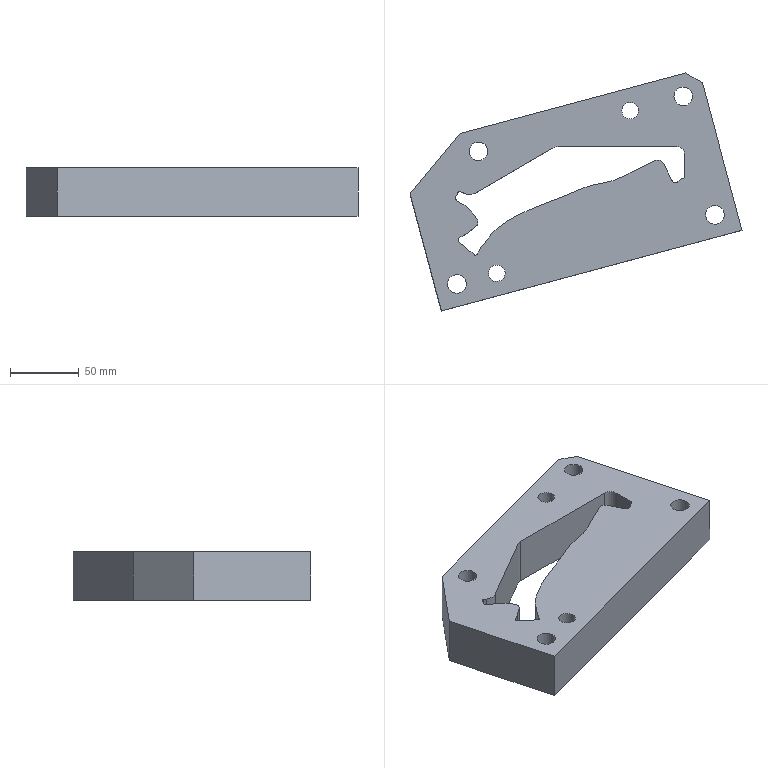Part | NX | features 7 2 | 1 solid | 67 faces | box 241.063 x 172.782 x 35 mm | volume 724957 mm3 | plane 30 | cylinder 21 | spline 16 | commonest cylinder face diameters 20 x5 13.5 x4 2 x3 3 x2 12.001 x2 14.11 x2